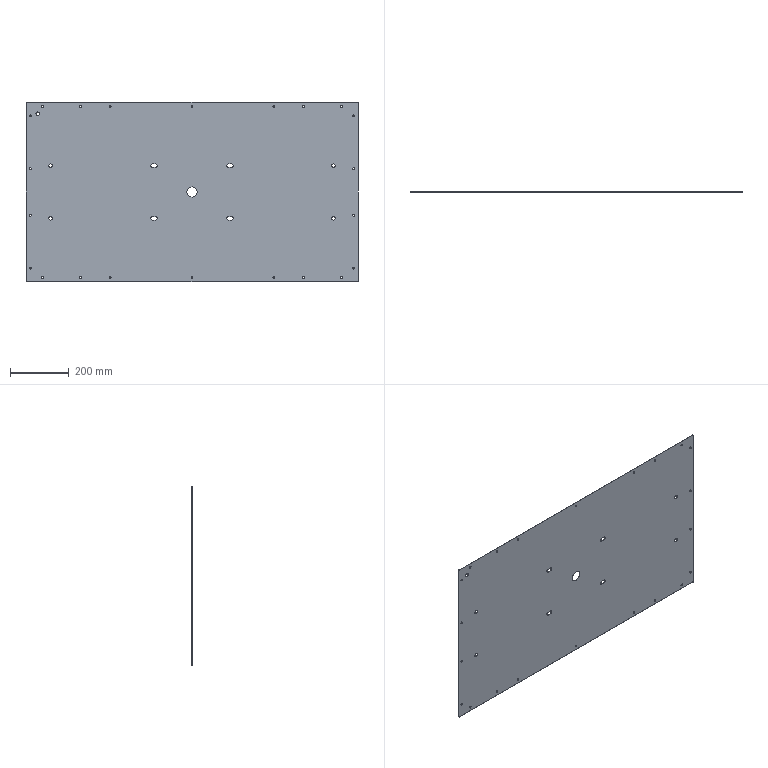Part | SolidWorks | features ICE 4, EdgeFlange 2, Fillet 1, FlatPattern 1, HoleWzd 1, SMBaseFlange 1, SheetMetal 1, WeldmentFeature 1 | 1 solid | 82 faces | box 1135 x 1.2 x 615 mm | volume 833766 mm3 | cylinder 68 | plane 14 | commonest cylinder face diameters 6.6 x44 12 x18 6 x4 35 x2